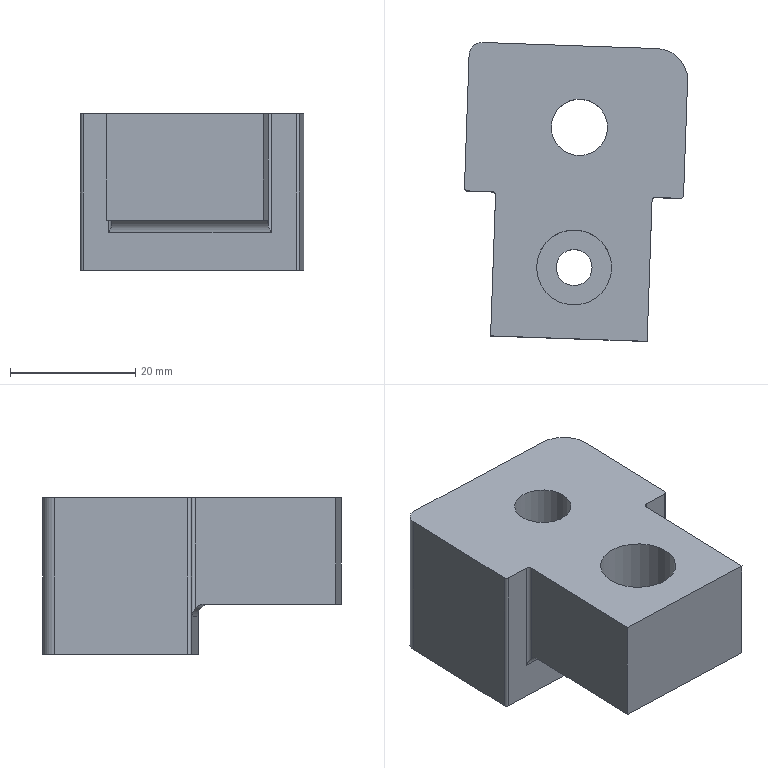Part | NX | features PS-28 2 | 1 solid | 23 faces | box 35.619 x 47.713 x 25 mm | volume 25847 mm3 | plane 12 | cylinder 11 | commonest cylinder face diameters 1 x4 4 x2 5.75 x1 9 x1 10 x1 12 x1
STEP:
#1=CARTESIAN_POINT('',(3329.391,-906.707,872.716));
#2=VERTEX_POINT('',#1);
#3=CARTESIAN_POINT('',(3332.266,-906.707,872.716));
#4=DIRECTION('',(0.,0.,-1.));
#5=DIRECTION('',(-1.,0.,0.));
#6=AXIS2_PLACEMENT_3D('',#3,#4,#5);
#7=CIRCLE('',#6,2.875);
#8=EDGE_CURVE('',#2,#2,#7,.F.);
#9=ORIENTED_EDGE('',*,*,#8,.T.);
#10=EDGE_LOOP('',(#9));
#11=FACE_BOUND('',#10,.T.);
#12=CARTESIAN_POINT('',(3329.391,-906.707,868.716));
#13=VERTEX_POINT('',#12);
#14=CARTESIAN_POINT('',(3332.266,-906.707,868.716));
#15=DIRECTION('',(0.,0.,-1.));
#16=DIRECTION('',(-1.,0.,0.));
#17=AXIS2_PLACEMENT_3D('',#14,#15,#16);
#18=CIRCLE('',#17,2.875);
#19=EDGE_CURVE('',#13,#13,#18,.F.);
#20=ORIENTED_EDGE('',*,*,#19,.F.);
#21=EDGE_LOOP('',(#20));
#22=FACE_BOUND('',#21,.T.);
#23=CARTESIAN_POINT('',(3332.266,-906.707,890.716));
#24=DIRECTION('',(0.,0.,-1.));
#25=DIRECTION('',(0.9976,-0.06975,0.));
#26=AXIS2_PLACEMENT_3D('',#23,#24,#25);
#27=CYLINDRICAL_SURFACE('',#26,2.875);
#28=ADVANCED_FACE('',(#11,#22),#27,.F.);
#29=CARTESIAN_POINT('',(3318.937,-917.63,885.716));
#30=VERTEX_POINT('',#29);
#31=CARTESIAN_POINT('',(3318.937,-917.63,868.716));
#32=VERTEX_POINT('',#31);
#33=CARTESIAN_POINT('',(3318.937,-917.63,863.216));
#34=DIRECTION('',(0.,0.,1.));
#35=VECTOR('',#34,1000.);
#36=LINE('',#33,#35);
#37=EDGE_CURVE('',#30,#32,#36,.F.);
#38=ORIENTED_EDGE('',*,*,#37,.F.);
#39=CARTESIAN_POINT('',(3319.722,-895.143,885.716));
#40=VERTEX_POINT('',#39);
#41=CARTESIAN_POINT('',(3319.52,-900.918,885.716));
#42=DIRECTION('',(0.0349,0.9994,0.));
#43=VECTOR('',#42,1000.);
#44=LINE('',#41,#43);
#45=EDGE_CURVE('',#30,#40,#44,.T.);
#46=ORIENTED_EDGE('',*,*,#45,.T.);
#47=CARTESIAN_POINT('',(3319.722,-895.143,868.039));
#48=VERTEX_POINT('',#47);
#49=CARTESIAN_POINT('',(3319.722,-895.143,868.716));
#50=DIRECTION('',(0.,0.,-1.));
#51=VECTOR('',#50,1000.);
#52=LINE('',#49,#51);
#53=EDGE_CURVE('',#40,#48,#52,.T.);
#54=ORIENTED_EDGE('',*,*,#53,.T.);
#55=CARTESIAN_POINT('',(3319.67,-896.642,868.716));
#56=VERTEX_POINT('',#55);
#57=CARTESIAN_POINT('',(3319.67,-896.642,866.716));
#58=DIRECTION('',(-0.9994,0.0349,0.));
#59=DIRECTION('',(-0.0349,-0.9994,0.));
#60=AXIS2_PLACEMENT_3D('',#57,#58,#59);
#61=CIRCLE('',#60,2.);
#62=EDGE_CURVE('',#56,#48,#61,.T.);
#63=ORIENTED_EDGE('',*,*,#62,.F.);
#64=CARTESIAN_POINT('',(3319.334,-906.255,868.716));
#65=DIRECTION('',(0.0349,0.9994,0.));
#66=VECTOR('',#65,1000.);
#67=LINE('',#64,#66);
#68=EDGE_CURVE('',#32,#56,#67,.T.);
#69=ORIENTED_EDGE('',*,*,#68,.F.);
#70=EDGE_LOOP('',(#38,#46,#54,#63,#69));
#71=FACE_BOUND('',#70,.T.);
#72=CARTESIAN_POINT('',(3319.52,-900.918,890.716));
#73=DIRECTION('',(0.9994,-0.0349,0.));
#74=DIRECTION('',(-0.0349,-0.9994,0.));
#75=AXIS2_PLACEMENT_3D('',#72,#73,#74);
#76=PLANE('',#75);
#77=ADVANCED_FACE('',(#71),#76,.F.);
#78=CARTESIAN_POINT('',(3343.922,-918.502,885.716));
#79=VERTEX_POINT('',#78);
#80=CARTESIAN_POINT('',(3328.742,-917.972,885.716));
#81=DIRECTION('',(-0.9994,0.0349,0.));
#82=VECTOR('',#81,1000.);
#83=LINE('',#80,#82);
#84=EDGE_CURVE('',#79,#30,#83,.T.);
#85=ORIENTED_EDGE('',*,*,#84,.T.);
#86=ORIENTED_EDGE('',*,*,#37,.T.);
#87=CARTESIAN_POINT('',(3343.922,-918.502,868.716));
#88=VERTEX_POINT('',#87);
#89=CARTESIAN_POINT('',(3328.742,-917.972,868.716));
#90=DIRECTION('',(0.9994,-0.0349,0.));
#91=VECTOR('',#90,1000.);
#92=LINE('',#89,#91);
#93=EDGE_CURVE('',#88,#32,#92,.F.);
#94=ORIENTED_EDGE('',*,*,#93,.F.);
#95=CARTESIAN_POINT('',(3343.922,-918.502,862.716));
#96=DIRECTION('',(0.,0.,-1.));
#97=VECTOR('',#96,1000.);
#98=LINE('',#95,#97);
#99=EDGE_CURVE('',#88,#79,#98,.F.);
#100=ORIENTED_EDGE('',*,*,#99,.T.);
#101=EDGE_LOOP('',(#85,#86,#94,#100));
#102=FACE_BOUND('',#101,.T.);
#103=CARTESIAN_POINT('',(3328.742,-917.972,863.216));
#104=DIRECTION('',(0.0349,0.9994,0.));
#105=DIRECTION('',(-0.9994,0.0349,0.));
#106=AXIS2_PLACEMENT_3D('',#103,#104,#105);
#107=PLANE('',#106);
#108=ADVANCED_FACE('',(#102),#107,.F.);
#109=CARTESIAN_POINT('',(3344.707,-896.016,885.716));
#110=VERTEX_POINT('',#109);
#111=CARTESIAN_POINT('',(3344.54,-900.791,885.716));
#112=DIRECTION('',(0.0349,0.9994,0.));
#113=VECTOR('',#112,1000.);
#114=LINE('',#111,#113);
#115=EDGE_CURVE('',#110,#79,#114,.F.);
#116=ORIENTED_EDGE('',*,*,#115,.T.);
#117=ORIENTED_EDGE('',*,*,#99,.F.);
#118=CARTESIAN_POINT('',(3344.654,-897.515,868.716));
#119=VERTEX_POINT('',#118);
#120=CARTESIAN_POINT('',(3344.319,-907.127,868.716));
#121=DIRECTION('',(0.0349,0.9994,0.));
#122=VECTOR('',#121,1000.);
#123=LINE('',#120,#122);
#124=EDGE_CURVE('',#88,#119,#123,.T.);
#125=ORIENTED_EDGE('',*,*,#124,.T.);
#126=CARTESIAN_POINT('',(3344.707,-896.016,868.039));
#127=VERTEX_POINT('',#126);
#128=CARTESIAN_POINT('',(3344.654,-897.515,866.716));
#129=DIRECTION('',(-0.9994,0.0349,0.));
#130=DIRECTION('',(-0.0349,-0.9994,0.));
#131=AXIS2_PLACEMENT_3D('',#128,#129,#130);
#132=CIRCLE('',#131,2.);
#133=EDGE_CURVE('',#127,#119,#132,.F.);
#134=ORIENTED_EDGE('',*,*,#133,.F.);
#135=CARTESIAN_POINT('',(3344.707,-896.016,862.716));
#136=DIRECTION('',(0.,0.,1.));
#137=VECTOR('',#136,1000.);
#138=LINE('',#135,#137);
#139=EDGE_CURVE('',#127,#110,#138,.T.);
#140=ORIENTED_EDGE('',*,*,#139,.T.);
#141=EDGE_LOOP('',(#116,#117,#125,#134,#140));
#142=FACE_BOUND('',#141,.T.);
#143=CARTESIAN_POINT('',(3344.54,-900.791,862.716));
#144=DIRECTION('',(0.9994,-0.0349,0.));
#145=DIRECTION('',(-0.0349,-0.9994,0.));
#146=AXIS2_PLACEMENT_3D('',#143,#144,#145);
#147=PLANE('',#146);
#148=ADVANCED_FACE('',(#142),#147,.T.);
#149=ORIENTED_EDGE('',*,*,#124,.F.);
#150=ORIENTED_EDGE('',*,*,#93,.T.);
#151=ORIENTED_EDGE('',*,*,#68,.T.);
#152=CARTESIAN_POINT('',(3332.601,-897.094,868.716));
#153=DIRECTION('',(0.9994,-0.0349,0.));
#154=VECTOR('',#153,1000.);
#155=LINE('',#152,#154);
#156=EDGE_CURVE('',#119,#56,#155,.F.);
#157=ORIENTED_EDGE('',*,*,#156,.F.);
#158=EDGE_LOOP('',(#149,#150,#151,#157));
#159=FACE_BOUND('',#158,.T.);
#160=ORIENTED_EDGE('',*,*,#19,.T.);
#161=EDGE_LOOP('',(#160));
#162=FACE_BOUND('',#161,.T.);
#163=CARTESIAN_POINT('',(3332.266,-906.707,868.716));
#164=DIRECTION('',(0.,0.,-1.));
#165=DIRECTION('',(-0.0349,-0.9994,0.));
#166=AXIS2_PLACEMENT_3D('',#163,#164,#165);
#167=PLANE('',#166);
#168=ADVANCED_FACE('',(#159,#162),#167,.T.);
#169=ORIENTED_EDGE('',*,*,#53,.F.);
#170=CARTESIAN_POINT('',(3319.24,-894.626,885.716));
#171=VERTEX_POINT('',#170);
#172=CARTESIAN_POINT('',(3319.222,-895.126,885.716));
#173=DIRECTION('',(0.,0.,-1.));
#174=DIRECTION('',(-1.,0.,0.));
#175=AXIS2_PLACEMENT_3D('',#172,#173,#174);
#176=CIRCLE('',#175,0.5);
#177=EDGE_CURVE('',#171,#40,#176,.T.);
#178=ORIENTED_EDGE('',*,*,#177,.F.);
#179=CARTESIAN_POINT('',(3319.24,-894.626,866.716));
#180=VERTEX_POINT('',#179);
#181=CARTESIAN_POINT('',(3319.24,-894.626,890.716));
#182=DIRECTION('',(0.,0.,-1.));
#183=VECTOR('',#182,1000.);
#184=LINE('',#181,#183);
#185=EDGE_CURVE('',#180,#171,#184,.F.);
#186=ORIENTED_EDGE('',*,*,#185,.F.);
#187=CARTESIAN_POINT('',(3319.722,-895.143,868.039));
#188=CARTESIAN_POINT('',(3319.734,-894.799,867.649));
#189=CARTESIAN_POINT('',(3319.469,-894.634,867.175));
#190=CARTESIAN_POINT('',(3319.24,-894.626,866.716));
#191=B_SPLINE_CURVE_WITH_KNOTS('',3,(#187,#188,#189,#190),.UNSPECIFIED.,.F.,.F.,(4,4),(0.,0.001539),.UNSPECIFIED.);
#192=EDGE_CURVE('',#48,#180,#191,.T.);
#193=ORIENTED_EDGE('',*,*,#192,.F.);
#194=EDGE_LOOP('',(#169,#178,#186,#193));
#195=FACE_BOUND('',#194,.T.);
#196=CARTESIAN_POINT('',(3319.222,-895.126,890.716));
#197=DIRECTION('',(0.,0.,1.));
#198=DIRECTION('',(1.,0.,0.));
#199=AXIS2_PLACEMENT_3D('',#196,#197,#198);
#200=CYLINDRICAL_SURFACE('',#199,0.5);
#201=ADVANCED_FACE('',(#195),#200,.F.);
#202=CARTESIAN_POINT('',(3345.224,-895.534,885.716));
#203=VERTEX_POINT('',#202);
#204=CARTESIAN_POINT('',(3345.224,-895.534,866.716));
#205=VERTEX_POINT('',#204);
#206=CARTESIAN_POINT('',(3345.224,-895.534,863.216));
#207=DIRECTION('',(0.,0.,1.));
#208=VECTOR('',#207,1000.);
#209=LINE('',#206,#208);
#210=EDGE_CURVE('',#203,#205,#209,.F.);
#211=ORIENTED_EDGE('',*,*,#210,.F.);
#212=CARTESIAN_POINT('',(3345.206,-896.033,885.716));
#213=DIRECTION('',(0.,0.,-1.));
#214=DIRECTION('',(-1.,0.,0.));
#215=AXIS2_PLACEMENT_3D('',#212,#213,#214);
#216=CIRCLE('',#215,0.5);
#217=EDGE_CURVE('',#203,#110,#216,.F.);
#218=ORIENTED_EDGE('',*,*,#217,.T.);
#219=ORIENTED_EDGE('',*,*,#139,.F.);
#220=CARTESIAN_POINT('',(3344.707,-896.016,868.039));
#221=CARTESIAN_POINT('',(3344.719,-895.672,867.649));
#222=CARTESIAN_POINT('',(3344.995,-895.526,867.175));
#223=CARTESIAN_POINT('',(3345.224,-895.534,866.716));
#224=B_SPLINE_CURVE_WITH_KNOTS('',3,(#220,#221,#222,#223),.UNSPECIFIED.,.F.,.F.,(4,4),(0.,0.001539),.UNSPECIFIED.);
#225=EDGE_CURVE('',#205,#127,#224,.F.);
#226=ORIENTED_EDGE('',*,*,#225,.F.);
#227=EDGE_LOOP('',(#211,#218,#219,#226));
#228=FACE_BOUND('',#227,.T.);
#229=CARTESIAN_POINT('',(3345.206,-896.033,862.716));
#230=DIRECTION('',(0.,0.,1.));
#231=DIRECTION('',(1.,0.,0.));
#232=AXIS2_PLACEMENT_3D('',#229,#230,#231);
#233=CYLINDRICAL_SURFACE('',#232,0.5);
#234=ADVANCED_FACE('',(#228),#233,.F.);
#235=CARTESIAN_POINT('',(3349.221,-895.673,860.716));
#236=VERTEX_POINT('',#235);
#237=CARTESIAN_POINT('',(3349.221,-895.673,885.716));
#238=VERTEX_POINT('',#237);
#239=CARTESIAN_POINT('',(3349.221,-895.673,890.716));
#240=DIRECTION('',(0.,0.,-1.));
#241=VECTOR('',#240,1000.);
#242=LINE('',#239,#241);
#243=EDGE_CURVE('',#236,#238,#242,.F.);
#244=ORIENTED_EDGE('',*,*,#243,.T.);
#245=CARTESIAN_POINT('',(3329.542,-894.986,885.716));
#246=DIRECTION('',(-0.9994,0.0349,0.));
#247=VECTOR('',#246,1000.);
#248=LINE('',#245,#247);
#249=EDGE_CURVE('',#203,#238,#248,.F.);
#250=ORIENTED_EDGE('',*,*,#249,.F.);
#251=ORIENTED_EDGE('',*,*,#210,.T.);
#252=CARTESIAN_POINT('',(3329.542,-894.986,866.716));
#253=DIRECTION('',(0.9994,-0.0349,0.));
#254=VECTOR('',#253,1000.);
#255=LINE('',#252,#254);
#256=EDGE_CURVE('',#180,#205,#255,.T.);
#257=ORIENTED_EDGE('',*,*,#256,.F.);
#258=ORIENTED_EDGE('',*,*,#185,.T.);
#259=CARTESIAN_POINT('',(3315.242,-894.487,885.716));
#260=VERTEX_POINT('',#259);
#261=CARTESIAN_POINT('',(3329.542,-894.986,885.716));
#262=DIRECTION('',(-0.9994,0.0349,0.));
#263=VECTOR('',#262,1000.);
#264=LINE('',#261,#263);
#265=EDGE_CURVE('',#260,#171,#264,.F.);
#266=ORIENTED_EDGE('',*,*,#265,.F.);
#267=CARTESIAN_POINT('',(3315.242,-894.487,860.716));
#268=VERTEX_POINT('',#267);
#269=CARTESIAN_POINT('',(3315.242,-894.487,863.216));
#270=DIRECTION('',(0.,0.,1.));
#271=VECTOR('',#270,1000.);
#272=LINE('',#269,#271);
#273=EDGE_CURVE('',#260,#268,#272,.F.);
#274=ORIENTED_EDGE('',*,*,#273,.T.);
#275=CARTESIAN_POINT('',(3329.542,-894.986,860.716));
#276=DIRECTION('',(-0.9994,0.0349,0.));
#277=VECTOR('',#276,1000.);
#278=LINE('',#275,#277);
#279=EDGE_CURVE('',#268,#236,#278,.F.);
#280=ORIENTED_EDGE('',*,*,#279,.T.);
#281=EDGE_LOOP('',(#244,#250,#251,#257,#258,#266,#274,#280));
#282=FACE_BOUND('',#281,.T.);
#283=CARTESIAN_POINT('',(3329.542,-894.986,863.216));
#284=DIRECTION('',(0.0349,0.9994,0.));
#285=DIRECTION('',(-0.9994,0.0349,0.));
#286=AXIS2_PLACEMENT_3D('',#283,#284,#285);
#287=PLANE('',#286);
#288=ADVANCED_FACE('',(#282),#287,.F.);
#289=CARTESIAN_POINT('',(3340.357,-884.341,860.716));
#290=VERTEX_POINT('',#289);
#291=CARTESIAN_POINT('',(3333.107,-884.341,860.716));
#292=DIRECTION('',(0.,0.,-1.));
#293=DIRECTION('',(1.,0.,0.));
#294=AXIS2_PLACEMENT_3D('',#291,#292,#293);
#295=CIRCLE('',#294,7.25);
#296=EDGE_CURVE('',#290,#290,#295,.T.);
#297=ORIENTED_EDGE('',*,*,#296,.F.);
#298=EDGE_LOOP('',(#297));
#299=FACE_BOUND('',#298,.T.);
#300=ORIENTED_EDGE('',*,*,#279,.F.);
#301=CARTESIAN_POINT('',(3314.76,-893.97,860.716));
#302=VERTEX_POINT('',#301);
#303=CARTESIAN_POINT('',(3315.26,-893.987,860.716));
#304=DIRECTION('',(0.,0.,-1.));
#305=DIRECTION('',(1.,0.,0.));
#306=AXIS2_PLACEMENT_3D('',#303,#304,#305);
#307=CIRCLE('',#306,0.5);
#308=EDGE_CURVE('',#268,#302,#307,.T.);
#309=ORIENTED_EDGE('',*,*,#308,.T.);
#310=CARTESIAN_POINT('',(3315.502,-872.719,860.716));
#311=VERTEX_POINT('',#310);
#312=CARTESIAN_POINT('',(3320.386,-732.845,860.716));
#313=DIRECTION('',(-0.0349,-0.9994,0.));
#314=VECTOR('',#313,1000.);
#315=LINE('',#312,#314);
#316=EDGE_CURVE('',#302,#311,#315,.F.);
#317=ORIENTED_EDGE('',*,*,#316,.T.);
#318=CARTESIAN_POINT('',(3317.57,-870.79,860.716));
#319=VERTEX_POINT('',#318);
#320=CARTESIAN_POINT('',(3317.501,-872.789,860.716));
#321=DIRECTION('',(0.,0.,-1.));
#322=DIRECTION('',(1.,0.,0.));
#323=AXIS2_PLACEMENT_3D('',#320,#321,#322);
#324=CIRCLE('',#323,2.);
#325=EDGE_CURVE('',#319,#311,#324,.F.);
#326=ORIENTED_EDGE('',*,*,#325,.F.);
#327=CARTESIAN_POINT('',(3345.553,-871.768,860.716));
#328=VERTEX_POINT('',#327);
#329=CARTESIAN_POINT('',(3304.578,-870.337,860.716));
#330=DIRECTION('',(0.9994,-0.0349,0.));
#331=VECTOR('',#330,1000.);
#332=LINE('',#329,#331);
#333=EDGE_CURVE('',#319,#328,#332,.T.);
#334=ORIENTED_EDGE('',*,*,#333,.T.);
#335=CARTESIAN_POINT('',(3350.376,-876.939,860.716));
#336=VERTEX_POINT('',#335);
#337=CARTESIAN_POINT('',(3345.379,-876.765,860.716));
#338=DIRECTION('',(0.,0.,-1.));
#339=DIRECTION('',(1.,0.,0.));
#340=AXIS2_PLACEMENT_3D('',#337,#338,#339);
#341=CIRCLE('',#340,5.);
#342=EDGE_CURVE('',#336,#328,#341,.F.);
#343=ORIENTED_EDGE('',*,*,#342,.F.);
#344=CARTESIAN_POINT('',(3349.739,-895.191,860.716));
#345=VERTEX_POINT('',#344);
#346=CARTESIAN_POINT('',(3355.365,-734.067,860.716));
#347=DIRECTION('',(-0.0349,-0.9994,0.));
#348=VECTOR('',#347,1000.);
#349=LINE('',#346,#348);
#350=EDGE_CURVE('',#345,#336,#349,.F.);
#351=ORIENTED_EDGE('',*,*,#350,.F.);
#352=CARTESIAN_POINT('',(3349.239,-895.173,860.716));
#353=DIRECTION('',(0.,0.,-1.));
#354=DIRECTION('',(1.,0.,0.));
#355=AXIS2_PLACEMENT_3D('',#352,#353,#354);
#356=CIRCLE('',#355,0.5);
#357=EDGE_CURVE('',#345,#236,#356,.T.);
#358=ORIENTED_EDGE('',*,*,#357,.T.);
#359=EDGE_LOOP('',(#300,#309,#317,#326,#334,#343,#351,#358));
#360=FACE_BOUND('',#359,.T.);
#361=CARTESIAN_POINT('',(2870.094,-717.123,860.716));
#362=DIRECTION('',(0.,0.,1.));
#363=DIRECTION('',(0.,-1.,0.));
#364=AXIS2_PLACEMENT_3D('',#361,#362,#363);
#365=PLANE('',#364);
#366=ADVANCED_FACE('',(#299,#360),#365,.F.);
#367=CARTESIAN_POINT('',(3349.739,-895.191,885.716));
#368=VERTEX_POINT('',#367);
#369=CARTESIAN_POINT('',(3350.376,-876.939,885.716));
#370=VERTEX_POINT('',#369);
#371=CARTESIAN_POINT('',(3349.537,-900.966,885.716));
#372=DIRECTION('',(0.0349,0.9994,0.));
#373=VECTOR('',#372,1000.);
#374=LINE('',#371,#373);
#375=EDGE_CURVE('',#368,#370,#374,.T.);
#376=ORIENTED_EDGE('',*,*,#375,.F.);
#377=CARTESIAN_POINT('',(3349.739,-895.191,868.716));
#378=DIRECTION('',(0.,0.,-1.));
#379=VECTOR('',#378,1000.);
#380=LINE('',#377,#379);
#381=EDGE_CURVE('',#368,#345,#380,.T.);
#382=ORIENTED_EDGE('',*,*,#381,.T.);
#383=ORIENTED_EDGE('',*,*,#350,.T.);
#384=CARTESIAN_POINT('',(3350.376,-876.939,862.716));
#385=DIRECTION('',(0.,0.,1.));
#386=VECTOR('',#385,1000.);
#387=LINE('',#384,#386);
#388=EDGE_CURVE('',#370,#336,#387,.F.);
#389=ORIENTED_EDGE('',*,*,#388,.F.);
#390=EDGE_LOOP('',(#376,#382,#383,#389));
#391=FACE_BOUND('',#390,.T.);
#392=CARTESIAN_POINT('',(3349.537,-900.966,862.716));
#393=DIRECTION('',(0.9994,-0.0349,0.));
#394=DIRECTION('',(-0.0349,-0.9994,0.));
#395=AXIS2_PLACEMENT_3D('',#392,#393,#394);
#396=PLANE('',#395);
#397=ADVANCED_FACE('',(#391),#396,.T.);
#398=CARTESIAN_POINT('',(3345.553,-871.768,885.716));
#399=VERTEX_POINT('',#398);
#400=CARTESIAN_POINT('',(3317.57,-870.79,885.716));
#401=VERTEX_POINT('',#400);
#402=CARTESIAN_POINT('',(3304.578,-870.337,885.716));
#403=DIRECTION('',(0.9994,-0.0349,0.));
#404=VECTOR('',#403,1000.);
#405=LINE('',#402,#404);
#406=EDGE_CURVE('',#399,#401,#405,.F.);
#407=ORIENTED_EDGE('',*,*,#406,.F.);
#408=CARTESIAN_POINT('',(3345.553,-871.768,935.716));
#409=DIRECTION('',(0.,0.,-1.));
#410=VECTOR('',#409,1000.);
#411=LINE('',#408,#410);
#412=EDGE_CURVE('',#328,#399,#411,.F.);
#413=ORIENTED_EDGE('',*,*,#412,.F.);
#414=ORIENTED_EDGE('',*,*,#333,.F.);
#415=CARTESIAN_POINT('',(3317.57,-870.79,860.716));
#416=DIRECTION('',(0.,0.,-1.));
#417=VECTOR('',#416,1000.);
#418=LINE('',#415,#417);
#419=EDGE_CURVE('',#401,#319,#418,.T.);
#420=ORIENTED_EDGE('',*,*,#419,.F.);
#421=EDGE_LOOP('',(#407,#413,#414,#420));
#422=FACE_BOUND('',#421,.T.);
#423=CARTESIAN_POINT('',(3304.578,-870.337,935.716));
#424=DIRECTION('',(-0.0349,-0.9994,0.));
#425=DIRECTION('',(-0.9994,0.0349,0.));
#426=AXIS2_PLACEMENT_3D('',#423,#424,#425);
#427=PLANE('',#426);
#428=ADVANCED_FACE('',(#422),#427,.F.);
#429=CARTESIAN_POINT('',(3314.76,-893.97,885.716));
#430=VERTEX_POINT('',#429);
#431=CARTESIAN_POINT('',(3314.76,-893.97,890.716));
#432=DIRECTION('',(0.,0.,1.));
#433=VECTOR('',#432,1000.);
#434=LINE('',#431,#433);
#435=EDGE_CURVE('',#302,#430,#434,.T.);
#436=ORIENTED_EDGE('',*,*,#435,.T.);
#437=CARTESIAN_POINT('',(3315.502,-872.719,885.716));
#438=VERTEX_POINT('',#437);
#439=CARTESIAN_POINT('',(3314.523,-900.744,885.716));
#440=DIRECTION('',(0.0349,0.9994,0.));
#441=VECTOR('',#440,1000.);
#442=LINE('',#439,#441);
#443=EDGE_CURVE('',#430,#438,#442,.T.);
#444=ORIENTED_EDGE('',*,*,#443,.T.);
#445=CARTESIAN_POINT('',(3315.502,-872.719,890.716));
#446=DIRECTION('',(0.,0.,1.));
#447=VECTOR('',#446,1000.);
#448=LINE('',#445,#447);
#449=EDGE_CURVE('',#311,#438,#448,.T.);
#450=ORIENTED_EDGE('',*,*,#449,.F.);
#451=ORIENTED_EDGE('',*,*,#316,.F.);
#452=EDGE_LOOP('',(#436,#444,#450,#451));
#453=FACE_BOUND('',#452,.T.);
#454=CARTESIAN_POINT('',(3314.523,-900.744,890.716));
#455=DIRECTION('',(0.9994,-0.0349,0.));
#456=DIRECTION('',(-0.0349,-0.9994,0.));
#457=AXIS2_PLACEMENT_3D('',#454,#455,#456);
#458=PLANE('',#457);
#459=ADVANCED_FACE('',(#453),#458,.F.);
#460=CARTESIAN_POINT('',(3317.501,-872.789,885.716));
#461=DIRECTION('',(0.,0.,-1.));
#462=DIRECTION('',(-1.,0.,0.));
#463=AXIS2_PLACEMENT_3D('',#460,#461,#462);
#464=CIRCLE('',#463,2.);
#465=EDGE_CURVE('',#438,#401,#464,.T.);
#466=ORIENTED_EDGE('',*,*,#465,.T.);
#467=ORIENTED_EDGE('',*,*,#419,.T.);
#468=ORIENTED_EDGE('',*,*,#325,.T.);
#469=ORIENTED_EDGE('',*,*,#449,.T.);
#470=EDGE_LOOP('',(#466,#467,#468,#469));
#471=FACE_BOUND('',#470,.T.);
#472=CARTESIAN_POINT('',(3317.501,-872.789,935.716));
#473=DIRECTION('',(0.,0.,-1.));
#474=DIRECTION('',(-0.9976,0.06975,0.));
#475=AXIS2_PLACEMENT_3D('',#472,#473,#474);
#476=CYLINDRICAL_SURFACE('',#475,2.);
#477=ADVANCED_FACE('',(#471),#476,.T.);
#478=CARTESIAN_POINT('',(3345.379,-876.765,885.716));
#479=DIRECTION('',(0.,0.,-1.));
#480=DIRECTION('',(-1.,0.,0.));
#481=AXIS2_PLACEMENT_3D('',#478,#479,#480);
#482=CIRCLE('',#481,5.);
#483=EDGE_CURVE('',#370,#399,#482,.F.);
#484=ORIENTED_EDGE('',*,*,#483,.F.);
#485=ORIENTED_EDGE('',*,*,#388,.T.);
#486=ORIENTED_EDGE('',*,*,#342,.T.);
#487=ORIENTED_EDGE('',*,*,#412,.T.);
#488=EDGE_LOOP('',(#484,#485,#486,#487));
#489=FACE_BOUND('',#488,.T.);
#490=CARTESIAN_POINT('',(3345.379,-876.765,862.716));
#491=DIRECTION('',(0.,0.,1.));
#492=DIRECTION('',(0.9976,-0.06975,0.));
#493=AXIS2_PLACEMENT_3D('',#490,#491,#492);
#494=CYLINDRICAL_SURFACE('',#493,5.);
#495=ADVANCED_FACE('',(#489),#494,.T.);
#496=CARTESIAN_POINT('',(3337.607,-884.341,874.716));
#497=VERTEX_POINT('',#496);
#498=CARTESIAN_POINT('',(3333.107,-884.341,874.716));
#499=DIRECTION('',(0.,0.,1.));
#500=DIRECTION('',(1.,0.,0.));
#501=AXIS2_PLACEMENT_3D('',#498,#499,#500);
#502=CIRCLE('',#501,4.5);
#503=EDGE_CURVE('',#497,#497,#502,.T.);
#504=ORIENTED_EDGE('',*,*,#503,.T.);
#505=EDGE_LOOP('',(#504));
#506=FACE_BOUND('',#505,.T.);
#507=CARTESIAN_POINT('',(3333.107,-891.591,874.716));
#508=VERTEX_POINT('',#507);
#509=CARTESIAN_POINT('',(3333.107,-884.341,874.716));
#510=DIRECTION('',(0.,0.,1.));
#511=DIRECTION('',(0.,-1.,0.));
#512=AXIS2_PLACEMENT_3D('',#509,#510,#511);
#513=CIRCLE('',#512,7.25);
#514=EDGE_CURVE('',#508,#508,#513,.F.);
#515=ORIENTED_EDGE('',*,*,#514,.T.);
#516=EDGE_LOOP('',(#515));
#517=FACE_BOUND('',#516,.T.);
#518=CARTESIAN_POINT('',(3333.107,-884.341,874.716));
#519=DIRECTION('',(0.,0.,1.));
#520=DIRECTION('',(0.9976,-0.06975,0.));
#521=AXIS2_PLACEMENT_3D('',#518,#519,#520);
#522=PLANE('',#521);
#523=ADVANCED_FACE('',(#506,#517),#522,.F.);
#524=ORIENTED_EDGE('',*,*,#514,.F.);
#525=EDGE_LOOP('',(#524));
#526=FACE_BOUND('',#525,.T.);
#527=ORIENTED_EDGE('',*,*,#296,.T.);
#528=EDGE_LOOP('',(#527));
#529=FACE_BOUND('',#528,.T.);
#530=CARTESIAN_POINT('',(3333.107,-884.341,868.716));
#531=DIRECTION('',(0.,0.,1.));
#532=DIRECTION('',(0.9976,-0.06975,0.));
#533=AXIS2_PLACEMENT_3D('',#530,#531,#532);
#534=CYLINDRICAL_SURFACE('',#533,7.25);
#535=ADVANCED_FACE('',(#526,#529),#534,.F.);
#536=CARTESIAN_POINT('',(3349.239,-895.173,885.716));
#537=DIRECTION('',(0.,0.,-1.));
#538=DIRECTION('',(-1.,0.,0.));
#539=AXIS2_PLACEMENT_3D('',#536,#537,#538);
#540=CIRCLE('',#539,0.5);
#541=EDGE_CURVE('',#238,#368,#540,.F.);
#542=ORIENTED_EDGE('',*,*,#541,.F.);
#543=ORIENTED_EDGE('',*,*,#243,.F.);
#544=ORIENTED_EDGE('',*,*,#357,.F.);
#545=ORIENTED_EDGE('',*,*,#381,.F.);
#546=EDGE_LOOP('',(#542,#543,#544,#545));
#547=FACE_BOUND('',#546,.T.);
#548=CARTESIAN_POINT('',(3349.239,-895.173,862.716));
#549=DIRECTION('',(0.,0.,1.));
#550=DIRECTION('',(1.,0.,0.));
#551=AXIS2_PLACEMENT_3D('',#548,#549,#550);
#552=CYLINDRICAL_SURFACE('',#551,0.5);
#553=ADVANCED_FACE('',(#547),#552,.T.);
#554=CARTESIAN_POINT('',(3315.26,-893.987,885.716));
#555=DIRECTION('',(0.,0.,-1.));
#556=DIRECTION('',(-1.,0.,0.));
#557=AXIS2_PLACEMENT_3D('',#554,#555,#556);
#558=CIRCLE('',#557,0.5);
#559=EDGE_CURVE('',#430,#260,#558,.F.);
#560=ORIENTED_EDGE('',*,*,#559,.F.);
#561=ORIENTED_EDGE('',*,*,#435,.F.);
#562=ORIENTED_EDGE('',*,*,#308,.F.);
#563=ORIENTED_EDGE('',*,*,#273,.F.);
#564=EDGE_LOOP('',(#560,#561,#562,#563));
#565=FACE_BOUND('',#564,.T.);
#566=CARTESIAN_POINT('',(3315.26,-893.987,890.716));
#567=DIRECTION('',(0.,0.,1.));
#568=DIRECTION('',(1.,0.,0.));
#569=AXIS2_PLACEMENT_3D('',#566,#567,#568);
#570=CYLINDRICAL_SURFACE('',#569,0.5);
#571=ADVANCED_FACE('',(#565),#570,.T.);
#572=ORIENTED_EDGE('',*,*,#62,.T.);
#573=ORIENTED_EDGE('',*,*,#192,.T.);
#574=ORIENTED_EDGE('',*,*,#256,.T.);
#575=ORIENTED_EDGE('',*,*,#225,.T.);
#576=ORIENTED_EDGE('',*,*,#133,.T.);
#577=ORIENTED_EDGE('',*,*,#156,.T.);
#578=EDGE_LOOP('',(#572,#573,#574,#575,#576,#577));
#579=FACE_BOUND('',#578,.T.);
#580=CARTESIAN_POINT('',(3329.472,-896.985,866.716));
#581=DIRECTION('',(0.9994,-0.0349,0.));
#582=DIRECTION('',(-0.0349,-0.9994,0.));
#583=AXIS2_PLACEMENT_3D('',#580,#581,#582);
#584=CYLINDRICAL_SURFACE('',#583,2.);
#585=ADVANCED_FACE('',(#579),#584,.F.);
#586=CARTESIAN_POINT('',(3328.607,-884.341,885.716));
#587=VERTEX_POINT('',#586);
#588=CARTESIAN_POINT('',(3333.107,-884.341,885.716));
#589=DIRECTION('',(0.,0.,-1.));
#590=DIRECTION('',(-1.,0.,0.));
#591=AXIS2_PLACEMENT_3D('',#588,#589,#590);
#592=CIRCLE('',#591,4.5);
#593=EDGE_CURVE('',#587,#587,#592,.T.);
#594=ORIENTED_EDGE('',*,*,#593,.T.);
#595=EDGE_LOOP('',(#594));
#596=FACE_BOUND('',#595,.T.);
#597=CARTESIAN_POINT('',(3326.266,-906.707,885.716));
#598=VERTEX_POINT('',#597);
#599=CARTESIAN_POINT('',(3332.266,-906.707,885.716));
#600=DIRECTION('',(0.,0.,-1.));
#601=DIRECTION('',(-1.,0.,0.));
#602=AXIS2_PLACEMENT_3D('',#599,#600,#601);
#603=CIRCLE('',#602,6.);
#604=EDGE_CURVE('',#598,#598,#603,.T.);
#605=ORIENTED_EDGE('',*,*,#604,.T.);
#606=EDGE_LOOP('',(#605));
#607=FACE_BOUND('',#606,.T.);
#608=ORIENTED_EDGE('',*,*,#249,.T.);
#609=ORIENTED_EDGE('',*,*,#541,.T.);
#610=ORIENTED_EDGE('',*,*,#375,.T.);
#611=ORIENTED_EDGE('',*,*,#483,.T.);
#612=ORIENTED_EDGE('',*,*,#406,.T.);
#613=ORIENTED_EDGE('',*,*,#465,.F.);
#614=ORIENTED_EDGE('',*,*,#443,.F.);
#615=ORIENTED_EDGE('',*,*,#559,.T.);
#616=ORIENTED_EDGE('',*,*,#265,.T.);
#617=ORIENTED_EDGE('',*,*,#177,.T.);
#618=ORIENTED_EDGE('',*,*,#45,.F.);
#619=ORIENTED_EDGE('',*,*,#84,.F.);
#620=ORIENTED_EDGE('',*,*,#115,.F.);
#621=ORIENTED_EDGE('',*,*,#217,.F.);
#622=EDGE_LOOP('',(#608,#609,#610,#611,#612,#613,#614,#615,#616,#617,#618,#619,#620,#621));
#623=FACE_BOUND('',#622,.T.);
#624=CARTESIAN_POINT('',(3332.569,-833.013,885.716));
#625=DIRECTION('',(0.,0.,-1.));
#626=DIRECTION('',(-1.,0.,0.));
#627=AXIS2_PLACEMENT_3D('',#624,#625,#626);
#628=PLANE('',#627);
#629=ADVANCED_FACE('',(#596,#607,#623),#628,.F.);
#630=CARTESIAN_POINT('',(3338.266,-906.707,872.716));
#631=VERTEX_POINT('',#630);
#632=CARTESIAN_POINT('',(3332.266,-906.707,872.716));
#633=DIRECTION('',(0.,0.,1.));
#634=DIRECTION('',(1.,0.,0.));
#635=AXIS2_PLACEMENT_3D('',#632,#633,#634);
#636=CIRCLE('',#635,6.);
#637=EDGE_CURVE('',#631,#631,#636,.F.);
#638=ORIENTED_EDGE('',*,*,#637,.F.);
#639=EDGE_LOOP('',(#638));
#640=FACE_BOUND('',#639,.T.);
#641=ORIENTED_EDGE('',*,*,#8,.F.);
#642=EDGE_LOOP('',(#641));
#643=FACE_BOUND('',#642,.T.);
#644=CARTESIAN_POINT('',(3332.266,-906.707,872.716));
#645=DIRECTION('',(0.,0.,-1.));
#646=DIRECTION('',(-1.,0.,0.));
#647=AXIS2_PLACEMENT_3D('',#644,#645,#646);
#648=PLANE('',#647);
#649=ADVANCED_FACE('',(#640,#643),#648,.F.);
#650=ORIENTED_EDGE('',*,*,#637,.T.);
#651=EDGE_LOOP('',(#650));
#652=FACE_BOUND('',#651,.T.);
#653=ORIENTED_EDGE('',*,*,#604,.F.);
#654=EDGE_LOOP('',(#653));
#655=FACE_BOUND('',#654,.T.);
#656=CARTESIAN_POINT('',(3332.266,-906.707,945.716));
#657=DIRECTION('',(0.,0.,-1.));
#658=DIRECTION('',(1.,0.,0.));
#659=AXIS2_PLACEMENT_3D('',#656,#657,#658);
#660=CYLINDRICAL_SURFACE('',#659,6.);
#661=ADVANCED_FACE('',(#652,#655),#660,.F.);
#662=ORIENTED_EDGE('',*,*,#503,.F.);
#663=EDGE_LOOP('',(#662));
#664=FACE_BOUND('',#663,.T.);
#665=ORIENTED_EDGE('',*,*,#593,.F.);
#666=EDGE_LOOP('',(#665));
#667=FACE_BOUND('',#666,.T.);
#668=CARTESIAN_POINT('',(3333.107,-884.341,874.716));
#669=DIRECTION('',(0.,0.,1.));
#670=DIRECTION('',(1.,0.,0.));
#671=AXIS2_PLACEMENT_3D('',#668,#669,#670);
#672=CYLINDRICAL_SURFACE('',#671,4.5);
#673=ADVANCED_FACE('',(#664,#667),#672,.F.);
#674=CLOSED_SHELL('',(#28,#77,#108,#148,#168,#201,#234,#288,#366,#397,#428,#459,#477,#495,#523,#535,#553,#571,#585,#629,#649,#661,#673));
#675=MANIFOLD_SOLID_BREP('',#674);
#676=(LENGTH_UNIT()NAMED_UNIT(*)SI_UNIT(.MILLI.,.METRE.));
#677=UNCERTAINTY_MEASURE_WITH_UNIT(LENGTH_MEASURE(0.0508),#676,'','');
#678=(NAMED_UNIT(*)PLANE_ANGLE_UNIT()SI_UNIT($,.RADIAN.));
#679=(NAMED_UNIT(*)SI_UNIT($,.STERADIAN.)SOLID_ANGLE_UNIT());
#680=(GEOMETRIC_REPRESENTATION_CONTEXT(3)GLOBAL_UNCERTAINTY_ASSIGNED_CONTEXT((#677))GLOBAL_UNIT_ASSIGNED_CONTEXT((#676,#678,#679))REPRESENTATION_CONTEXT('',''));
#681=ADVANCED_BREP_SHAPE_REPRESENTATION('',(#675),#680);